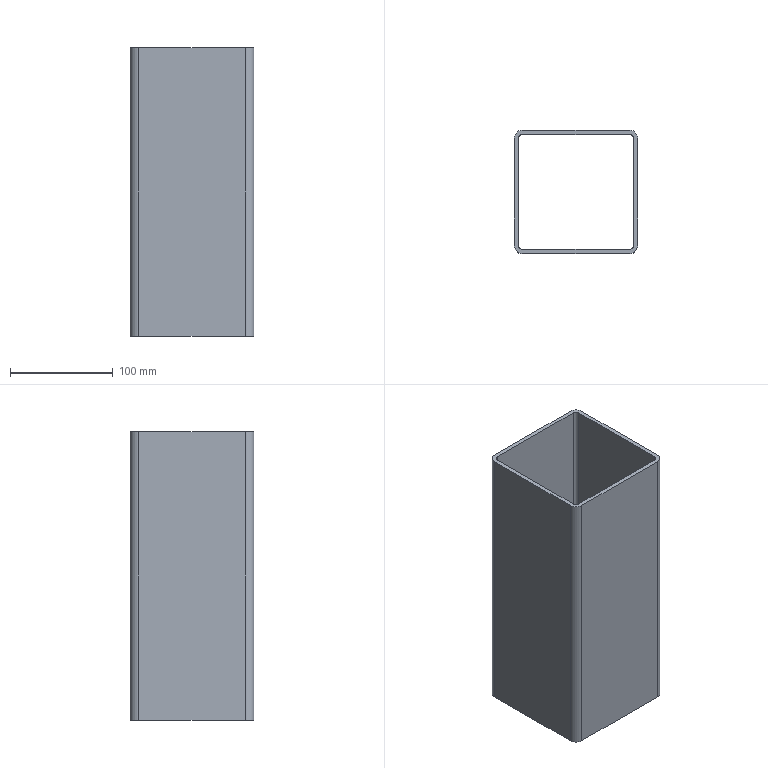Part | SolidWorks | features ICE 1, LibraryFeature 1 | 1 solid | 18 faces | box 120 x 120 x 280 mm | volume 508143 mm3 | plane 10 | cylinder 8 | commonest cylinder face diameters 8 x4 16 x4
STEP:
#1=CARTESIAN_POINT('',(52.,60.,-140.));
#2=VERTEX_POINT('',#1);
#3=CARTESIAN_POINT('',(-52.,60.,-140.));
#4=VERTEX_POINT('',#3);
#5=CARTESIAN_POINT('',(0.,60.,-140.));
#6=DIRECTION('',(-1.,0.,0.));
#7=VECTOR('',#6,1000.);
#8=LINE('',#5,#7);
#9=EDGE_CURVE('',#2,#4,#8,.T.);
#10=ORIENTED_EDGE('',*,*,#9,.T.);
#11=CARTESIAN_POINT('',(-52.,60.,140.));
#12=VERTEX_POINT('',#11);
#13=CARTESIAN_POINT('',(-52.,60.,140.));
#14=DIRECTION('',(0.,0.,-1.));
#15=VECTOR('',#14,1000.);
#16=LINE('',#13,#15);
#17=EDGE_CURVE('',#12,#4,#16,.T.);
#18=ORIENTED_EDGE('',*,*,#17,.F.);
#19=CARTESIAN_POINT('',(52.,60.,140.));
#20=VERTEX_POINT('',#19);
#21=CARTESIAN_POINT('',(0.,60.,140.));
#22=DIRECTION('',(-1.,0.,0.));
#23=VECTOR('',#22,1000.);
#24=LINE('',#21,#23);
#25=EDGE_CURVE('',#20,#12,#24,.T.);
#26=ORIENTED_EDGE('',*,*,#25,.F.);
#27=CARTESIAN_POINT('',(52.,60.,140.));
#28=DIRECTION('',(0.,0.,-1.));
#29=VECTOR('',#28,1000.);
#30=LINE('',#27,#29);
#31=EDGE_CURVE('',#20,#2,#30,.T.);
#32=ORIENTED_EDGE('',*,*,#31,.T.);
#33=EDGE_LOOP('',(#10,#18,#26,#32));
#34=FACE_OUTER_BOUND('',#33,.T.);
#35=CARTESIAN_POINT('',(0.,60.,140.));
#36=DIRECTION('',(0.,-1.,0.));
#37=DIRECTION('',(0.,0.,-1.));
#38=AXIS2_PLACEMENT_3D('',#35,#36,#37);
#39=PLANE('',#38);
#40=ADVANCED_FACE('',(#34),#39,.F.);
#41=CARTESIAN_POINT('',(-60.,52.,-140.));
#42=VERTEX_POINT('',#41);
#43=CARTESIAN_POINT('',(-52.,52.,-140.));
#44=DIRECTION('',(0.,0.,1.));
#45=DIRECTION('',(1.,0.,0.));
#46=AXIS2_PLACEMENT_3D('',#43,#44,#45);
#47=CIRCLE('',#46,8.);
#48=EDGE_CURVE('',#4,#42,#47,.T.);
#49=ORIENTED_EDGE('',*,*,#48,.T.);
#50=CARTESIAN_POINT('',(-60.,52.,140.));
#51=VERTEX_POINT('',#50);
#52=CARTESIAN_POINT('',(-60.,52.,140.));
#53=DIRECTION('',(0.,0.,-1.));
#54=VECTOR('',#53,1000.);
#55=LINE('',#52,#54);
#56=EDGE_CURVE('',#51,#42,#55,.T.);
#57=ORIENTED_EDGE('',*,*,#56,.F.);
#58=CARTESIAN_POINT('',(-52.,52.,140.));
#59=DIRECTION('',(0.,0.,1.));
#60=DIRECTION('',(1.,0.,0.));
#61=AXIS2_PLACEMENT_3D('',#58,#59,#60);
#62=CIRCLE('',#61,8.);
#63=EDGE_CURVE('',#12,#51,#62,.T.);
#64=ORIENTED_EDGE('',*,*,#63,.F.);
#65=ORIENTED_EDGE('',*,*,#17,.T.);
#66=EDGE_LOOP('',(#49,#57,#64,#65));
#67=FACE_OUTER_BOUND('',#66,.T.);
#68=CARTESIAN_POINT('',(-52.,52.,140.));
#69=DIRECTION('',(0.,0.,-1.));
#70=DIRECTION('',(-1.,0.,0.));
#71=AXIS2_PLACEMENT_3D('',#68,#69,#70);
#72=CYLINDRICAL_SURFACE('',#71,8.);
#73=ADVANCED_FACE('',(#67),#72,.T.);
#74=CARTESIAN_POINT('',(-60.,-52.,-140.));
#75=VERTEX_POINT('',#74);
#76=CARTESIAN_POINT('',(-60.,0.,-140.));
#77=DIRECTION('',(0.,1.,0.));
#78=VECTOR('',#77,1000.);
#79=LINE('',#76,#78);
#80=EDGE_CURVE('',#75,#42,#79,.T.);
#81=ORIENTED_EDGE('',*,*,#80,.F.);
#82=CARTESIAN_POINT('',(-60.,-52.,140.));
#83=VERTEX_POINT('',#82);
#84=CARTESIAN_POINT('',(-60.,-52.,140.));
#85=DIRECTION('',(0.,0.,-1.));
#86=VECTOR('',#85,1000.);
#87=LINE('',#84,#86);
#88=EDGE_CURVE('',#83,#75,#87,.T.);
#89=ORIENTED_EDGE('',*,*,#88,.F.);
#90=CARTESIAN_POINT('',(-60.,0.,140.));
#91=DIRECTION('',(0.,1.,0.));
#92=VECTOR('',#91,1000.);
#93=LINE('',#90,#92);
#94=EDGE_CURVE('',#83,#51,#93,.T.);
#95=ORIENTED_EDGE('',*,*,#94,.T.);
#96=ORIENTED_EDGE('',*,*,#56,.T.);
#97=EDGE_LOOP('',(#81,#89,#95,#96));
#98=FACE_OUTER_BOUND('',#97,.T.);
#99=CARTESIAN_POINT('',(-60.,0.,140.));
#100=DIRECTION('',(-1.,0.,0.));
#101=DIRECTION('',(0.,0.,1.));
#102=AXIS2_PLACEMENT_3D('',#99,#100,#101);
#103=PLANE('',#102);
#104=ADVANCED_FACE('',(#98),#103,.T.);
#105=CARTESIAN_POINT('',(-52.,-60.,-140.));
#106=VERTEX_POINT('',#105);
#107=CARTESIAN_POINT('',(-52.,-52.,-140.));
#108=DIRECTION('',(0.,0.,1.));
#109=DIRECTION('',(1.,0.,0.));
#110=AXIS2_PLACEMENT_3D('',#107,#108,#109);
#111=CIRCLE('',#110,8.);
#112=EDGE_CURVE('',#75,#106,#111,.T.);
#113=ORIENTED_EDGE('',*,*,#112,.T.);
#114=CARTESIAN_POINT('',(-52.,-60.,140.));
#115=VERTEX_POINT('',#114);
#116=CARTESIAN_POINT('',(-52.,-60.,140.));
#117=DIRECTION('',(0.,0.,-1.));
#118=VECTOR('',#117,1000.);
#119=LINE('',#116,#118);
#120=EDGE_CURVE('',#115,#106,#119,.T.);
#121=ORIENTED_EDGE('',*,*,#120,.F.);
#122=CARTESIAN_POINT('',(-52.,-52.,140.));
#123=DIRECTION('',(0.,0.,1.));
#124=DIRECTION('',(1.,0.,0.));
#125=AXIS2_PLACEMENT_3D('',#122,#123,#124);
#126=CIRCLE('',#125,8.);
#127=EDGE_CURVE('',#83,#115,#126,.T.);
#128=ORIENTED_EDGE('',*,*,#127,.F.);
#129=ORIENTED_EDGE('',*,*,#88,.T.);
#130=EDGE_LOOP('',(#113,#121,#128,#129));
#131=FACE_OUTER_BOUND('',#130,.T.);
#132=CARTESIAN_POINT('',(-52.,-52.,140.));
#133=DIRECTION('',(0.,0.,-1.));
#134=DIRECTION('',(-1.,0.,0.));
#135=AXIS2_PLACEMENT_3D('',#132,#133,#134);
#136=CYLINDRICAL_SURFACE('',#135,8.);
#137=ADVANCED_FACE('',(#131),#136,.T.);
#138=CARTESIAN_POINT('',(52.,-60.,-140.));
#139=VERTEX_POINT('',#138);
#140=CARTESIAN_POINT('',(0.,-60.,-140.));
#141=DIRECTION('',(1.,0.,0.));
#142=VECTOR('',#141,1000.);
#143=LINE('',#140,#142);
#144=EDGE_CURVE('',#106,#139,#143,.T.);
#145=ORIENTED_EDGE('',*,*,#144,.T.);
#146=CARTESIAN_POINT('',(52.,-60.,140.));
#147=VERTEX_POINT('',#146);
#148=CARTESIAN_POINT('',(52.,-60.,140.));
#149=DIRECTION('',(0.,0.,-1.));
#150=VECTOR('',#149,1000.);
#151=LINE('',#148,#150);
#152=EDGE_CURVE('',#147,#139,#151,.T.);
#153=ORIENTED_EDGE('',*,*,#152,.F.);
#154=CARTESIAN_POINT('',(0.,-60.,140.));
#155=DIRECTION('',(1.,0.,0.));
#156=VECTOR('',#155,1000.);
#157=LINE('',#154,#156);
#158=EDGE_CURVE('',#115,#147,#157,.T.);
#159=ORIENTED_EDGE('',*,*,#158,.F.);
#160=ORIENTED_EDGE('',*,*,#120,.T.);
#161=EDGE_LOOP('',(#145,#153,#159,#160));
#162=FACE_OUTER_BOUND('',#161,.T.);
#163=CARTESIAN_POINT('',(0.,-60.,140.));
#164=DIRECTION('',(0.,1.,0.));
#165=DIRECTION('',(0.,0.,1.));
#166=AXIS2_PLACEMENT_3D('',#163,#164,#165);
#167=PLANE('',#166);
#168=ADVANCED_FACE('',(#162),#167,.F.);
#169=CARTESIAN_POINT('',(60.,-52.,-140.));
#170=VERTEX_POINT('',#169);
#171=CARTESIAN_POINT('',(52.,-52.,-140.));
#172=DIRECTION('',(0.,0.,1.));
#173=DIRECTION('',(1.,0.,0.));
#174=AXIS2_PLACEMENT_3D('',#171,#172,#173);
#175=CIRCLE('',#174,8.);
#176=EDGE_CURVE('',#139,#170,#175,.T.);
#177=ORIENTED_EDGE('',*,*,#176,.T.);
#178=CARTESIAN_POINT('',(60.,-52.,140.));
#179=VERTEX_POINT('',#178);
#180=CARTESIAN_POINT('',(60.,-52.,140.));
#181=DIRECTION('',(0.,0.,-1.));
#182=VECTOR('',#181,1000.);
#183=LINE('',#180,#182);
#184=EDGE_CURVE('',#179,#170,#183,.T.);
#185=ORIENTED_EDGE('',*,*,#184,.F.);
#186=CARTESIAN_POINT('',(52.,-52.,140.));
#187=DIRECTION('',(0.,0.,1.));
#188=DIRECTION('',(1.,0.,0.));
#189=AXIS2_PLACEMENT_3D('',#186,#187,#188);
#190=CIRCLE('',#189,8.);
#191=EDGE_CURVE('',#147,#179,#190,.T.);
#192=ORIENTED_EDGE('',*,*,#191,.F.);
#193=ORIENTED_EDGE('',*,*,#152,.T.);
#194=EDGE_LOOP('',(#177,#185,#192,#193));
#195=FACE_OUTER_BOUND('',#194,.T.);
#196=CARTESIAN_POINT('',(52.,-52.,140.));
#197=DIRECTION('',(0.,0.,-1.));
#198=DIRECTION('',(-1.,0.,0.));
#199=AXIS2_PLACEMENT_3D('',#196,#197,#198);
#200=CYLINDRICAL_SURFACE('',#199,8.);
#201=ADVANCED_FACE('',(#195),#200,.T.);
#202=CARTESIAN_POINT('',(60.,52.,-140.));
#203=VERTEX_POINT('',#202);
#204=CARTESIAN_POINT('',(60.,0.,-140.));
#205=DIRECTION('',(0.,-1.,0.));
#206=VECTOR('',#205,1000.);
#207=LINE('',#204,#206);
#208=EDGE_CURVE('',#203,#170,#207,.T.);
#209=ORIENTED_EDGE('',*,*,#208,.F.);
#210=CARTESIAN_POINT('',(60.,52.,140.));
#211=VERTEX_POINT('',#210);
#212=CARTESIAN_POINT('',(60.,52.,140.));
#213=DIRECTION('',(0.,0.,-1.));
#214=VECTOR('',#213,1000.);
#215=LINE('',#212,#214);
#216=EDGE_CURVE('',#211,#203,#215,.T.);
#217=ORIENTED_EDGE('',*,*,#216,.F.);
#218=CARTESIAN_POINT('',(60.,0.,140.));
#219=DIRECTION('',(0.,-1.,0.));
#220=VECTOR('',#219,1000.);
#221=LINE('',#218,#220);
#222=EDGE_CURVE('',#211,#179,#221,.T.);
#223=ORIENTED_EDGE('',*,*,#222,.T.);
#224=ORIENTED_EDGE('',*,*,#184,.T.);
#225=EDGE_LOOP('',(#209,#217,#223,#224));
#226=FACE_OUTER_BOUND('',#225,.T.);
#227=CARTESIAN_POINT('',(60.,0.,140.));
#228=DIRECTION('',(1.,0.,0.));
#229=DIRECTION('',(0.,0.,-1.));
#230=AXIS2_PLACEMENT_3D('',#227,#228,#229);
#231=PLANE('',#230);
#232=ADVANCED_FACE('',(#226),#231,.T.);
#233=CARTESIAN_POINT('',(-56.,-52.,-140.));
#234=VERTEX_POINT('',#233);
#235=CARTESIAN_POINT('',(-52.,-56.,-140.));
#236=VERTEX_POINT('',#235);
#237=CARTESIAN_POINT('',(-52.,-52.,-140.));
#238=DIRECTION('',(0.,0.,1.));
#239=DIRECTION('',(1.,0.,0.));
#240=AXIS2_PLACEMENT_3D('',#237,#238,#239);
#241=CIRCLE('',#240,4.);
#242=EDGE_CURVE('',#234,#236,#241,.T.);
#243=ORIENTED_EDGE('',*,*,#242,.F.);
#244=CARTESIAN_POINT('',(-56.,-52.,140.));
#245=VERTEX_POINT('',#244);
#246=CARTESIAN_POINT('',(-56.,-52.,140.));
#247=DIRECTION('',(0.,0.,-1.));
#248=VECTOR('',#247,1000.);
#249=LINE('',#246,#248);
#250=EDGE_CURVE('',#245,#234,#249,.T.);
#251=ORIENTED_EDGE('',*,*,#250,.F.);
#252=CARTESIAN_POINT('',(-52.,-56.,140.));
#253=VERTEX_POINT('',#252);
#254=CARTESIAN_POINT('',(-52.,-52.,140.));
#255=DIRECTION('',(0.,0.,1.));
#256=DIRECTION('',(1.,0.,0.));
#257=AXIS2_PLACEMENT_3D('',#254,#255,#256);
#258=CIRCLE('',#257,4.);
#259=EDGE_CURVE('',#245,#253,#258,.T.);
#260=ORIENTED_EDGE('',*,*,#259,.T.);
#261=CARTESIAN_POINT('',(-52.,-56.,140.));
#262=DIRECTION('',(0.,0.,-1.));
#263=VECTOR('',#262,1000.);
#264=LINE('',#261,#263);
#265=EDGE_CURVE('',#253,#236,#264,.T.);
#266=ORIENTED_EDGE('',*,*,#265,.T.);
#267=EDGE_LOOP('',(#243,#251,#260,#266));
#268=FACE_OUTER_BOUND('',#267,.T.);
#269=CARTESIAN_POINT('',(-52.,-52.,140.));
#270=DIRECTION('',(0.,0.,-1.));
#271=DIRECTION('',(-1.,0.,0.));
#272=AXIS2_PLACEMENT_3D('',#269,#270,#271);
#273=CYLINDRICAL_SURFACE('',#272,4.);
#274=ADVANCED_FACE('',(#268),#273,.F.);
#275=CARTESIAN_POINT('',(-56.,52.,-140.));
#276=VERTEX_POINT('',#275);
#277=CARTESIAN_POINT('',(-56.,0.,-140.));
#278=DIRECTION('',(0.,1.,0.));
#279=VECTOR('',#278,1000.);
#280=LINE('',#277,#279);
#281=EDGE_CURVE('',#234,#276,#280,.T.);
#282=ORIENTED_EDGE('',*,*,#281,.T.);
#283=CARTESIAN_POINT('',(-56.,52.,140.));
#284=VERTEX_POINT('',#283);
#285=CARTESIAN_POINT('',(-56.,52.,140.));
#286=DIRECTION('',(0.,0.,-1.));
#287=VECTOR('',#286,1000.);
#288=LINE('',#285,#287);
#289=EDGE_CURVE('',#284,#276,#288,.T.);
#290=ORIENTED_EDGE('',*,*,#289,.F.);
#291=CARTESIAN_POINT('',(-56.,0.,140.));
#292=DIRECTION('',(0.,1.,0.));
#293=VECTOR('',#292,1000.);
#294=LINE('',#291,#293);
#295=EDGE_CURVE('',#245,#284,#294,.T.);
#296=ORIENTED_EDGE('',*,*,#295,.F.);
#297=ORIENTED_EDGE('',*,*,#250,.T.);
#298=EDGE_LOOP('',(#282,#290,#296,#297));
#299=FACE_OUTER_BOUND('',#298,.T.);
#300=CARTESIAN_POINT('',(-56.,0.,140.));
#301=DIRECTION('',(-1.,0.,0.));
#302=DIRECTION('',(0.,0.,1.));
#303=AXIS2_PLACEMENT_3D('',#300,#301,#302);
#304=PLANE('',#303);
#305=ADVANCED_FACE('',(#299),#304,.F.);
#306=CARTESIAN_POINT('',(-52.,56.,-140.));
#307=VERTEX_POINT('',#306);
#308=CARTESIAN_POINT('',(-52.,52.,-140.));
#309=DIRECTION('',(0.,0.,1.));
#310=DIRECTION('',(1.,0.,0.));
#311=AXIS2_PLACEMENT_3D('',#308,#309,#310);
#312=CIRCLE('',#311,4.);
#313=EDGE_CURVE('',#307,#276,#312,.T.);
#314=ORIENTED_EDGE('',*,*,#313,.F.);
#315=CARTESIAN_POINT('',(-52.,56.,140.));
#316=VERTEX_POINT('',#315);
#317=CARTESIAN_POINT('',(-52.,56.,140.));
#318=DIRECTION('',(0.,0.,-1.));
#319=VECTOR('',#318,1000.);
#320=LINE('',#317,#319);
#321=EDGE_CURVE('',#316,#307,#320,.T.);
#322=ORIENTED_EDGE('',*,*,#321,.F.);
#323=CARTESIAN_POINT('',(-52.,52.,140.));
#324=DIRECTION('',(0.,0.,1.));
#325=DIRECTION('',(1.,0.,0.));
#326=AXIS2_PLACEMENT_3D('',#323,#324,#325);
#327=CIRCLE('',#326,4.);
#328=EDGE_CURVE('',#316,#284,#327,.T.);
#329=ORIENTED_EDGE('',*,*,#328,.T.);
#330=ORIENTED_EDGE('',*,*,#289,.T.);
#331=EDGE_LOOP('',(#314,#322,#329,#330));
#332=FACE_OUTER_BOUND('',#331,.T.);
#333=CARTESIAN_POINT('',(-52.,52.,140.));
#334=DIRECTION('',(0.,0.,-1.));
#335=DIRECTION('',(-1.,0.,0.));
#336=AXIS2_PLACEMENT_3D('',#333,#334,#335);
#337=CYLINDRICAL_SURFACE('',#336,4.);
#338=ADVANCED_FACE('',(#332),#337,.F.);
#339=CARTESIAN_POINT('',(52.,56.,-140.));
#340=VERTEX_POINT('',#339);
#341=CARTESIAN_POINT('',(0.,56.,-140.));
#342=DIRECTION('',(-1.,0.,0.));
#343=VECTOR('',#342,1000.);
#344=LINE('',#341,#343);
#345=EDGE_CURVE('',#340,#307,#344,.T.);
#346=ORIENTED_EDGE('',*,*,#345,.F.);
#347=CARTESIAN_POINT('',(52.,56.,140.));
#348=VERTEX_POINT('',#347);
#349=CARTESIAN_POINT('',(52.,56.,140.));
#350=DIRECTION('',(0.,0.,-1.));
#351=VECTOR('',#350,1000.);
#352=LINE('',#349,#351);
#353=EDGE_CURVE('',#348,#340,#352,.T.);
#354=ORIENTED_EDGE('',*,*,#353,.F.);
#355=CARTESIAN_POINT('',(0.,56.,140.));
#356=DIRECTION('',(-1.,0.,0.));
#357=VECTOR('',#356,1000.);
#358=LINE('',#355,#357);
#359=EDGE_CURVE('',#348,#316,#358,.T.);
#360=ORIENTED_EDGE('',*,*,#359,.T.);
#361=ORIENTED_EDGE('',*,*,#321,.T.);
#362=EDGE_LOOP('',(#346,#354,#360,#361));
#363=FACE_OUTER_BOUND('',#362,.T.);
#364=CARTESIAN_POINT('',(0.,56.,140.));
#365=DIRECTION('',(0.,-1.,0.));
#366=DIRECTION('',(0.,0.,-1.));
#367=AXIS2_PLACEMENT_3D('',#364,#365,#366);
#368=PLANE('',#367);
#369=ADVANCED_FACE('',(#363),#368,.T.);
#370=CARTESIAN_POINT('',(56.,52.,-140.));
#371=VERTEX_POINT('',#370);
#372=CARTESIAN_POINT('',(52.,52.,-140.));
#373=DIRECTION('',(0.,0.,1.));
#374=DIRECTION('',(1.,0.,0.));
#375=AXIS2_PLACEMENT_3D('',#372,#373,#374);
#376=CIRCLE('',#375,4.);
#377=EDGE_CURVE('',#371,#340,#376,.T.);
#378=ORIENTED_EDGE('',*,*,#377,.F.);
#379=CARTESIAN_POINT('',(56.,52.,140.));
#380=VERTEX_POINT('',#379);
#381=CARTESIAN_POINT('',(56.,52.,140.));
#382=DIRECTION('',(0.,0.,-1.));
#383=VECTOR('',#382,1000.);
#384=LINE('',#381,#383);
#385=EDGE_CURVE('',#380,#371,#384,.T.);
#386=ORIENTED_EDGE('',*,*,#385,.F.);
#387=CARTESIAN_POINT('',(52.,52.,140.));
#388=DIRECTION('',(0.,0.,1.));
#389=DIRECTION('',(1.,0.,0.));
#390=AXIS2_PLACEMENT_3D('',#387,#388,#389);
#391=CIRCLE('',#390,4.);
#392=EDGE_CURVE('',#380,#348,#391,.T.);
#393=ORIENTED_EDGE('',*,*,#392,.T.);
#394=ORIENTED_EDGE('',*,*,#353,.T.);
#395=EDGE_LOOP('',(#378,#386,#393,#394));
#396=FACE_OUTER_BOUND('',#395,.T.);
#397=CARTESIAN_POINT('',(52.,52.,140.));
#398=DIRECTION('',(0.,0.,-1.));
#399=DIRECTION('',(-1.,0.,0.));
#400=AXIS2_PLACEMENT_3D('',#397,#398,#399);
#401=CYLINDRICAL_SURFACE('',#400,4.);
#402=ADVANCED_FACE('',(#396),#401,.F.);
#403=CARTESIAN_POINT('',(56.,-52.,-140.));
#404=VERTEX_POINT('',#403);
#405=CARTESIAN_POINT('',(56.,0.,-140.));
#406=DIRECTION('',(0.,-1.,0.));
#407=VECTOR('',#406,1000.);
#408=LINE('',#405,#407);
#409=EDGE_CURVE('',#371,#404,#408,.T.);
#410=ORIENTED_EDGE('',*,*,#409,.T.);
#411=CARTESIAN_POINT('',(56.,-52.,140.));
#412=VERTEX_POINT('',#411);
#413=CARTESIAN_POINT('',(56.,-52.,140.));
#414=DIRECTION('',(0.,0.,-1.));
#415=VECTOR('',#414,1000.);
#416=LINE('',#413,#415);
#417=EDGE_CURVE('',#412,#404,#416,.T.);
#418=ORIENTED_EDGE('',*,*,#417,.F.);
#419=CARTESIAN_POINT('',(56.,0.,140.));
#420=DIRECTION('',(0.,-1.,0.));
#421=VECTOR('',#420,1000.);
#422=LINE('',#419,#421);
#423=EDGE_CURVE('',#380,#412,#422,.T.);
#424=ORIENTED_EDGE('',*,*,#423,.F.);
#425=ORIENTED_EDGE('',*,*,#385,.T.);
#426=EDGE_LOOP('',(#410,#418,#424,#425));
#427=FACE_OUTER_BOUND('',#426,.T.);
#428=CARTESIAN_POINT('',(56.,0.,140.));
#429=DIRECTION('',(1.,0.,0.));
#430=DIRECTION('',(0.,0.,-1.));
#431=AXIS2_PLACEMENT_3D('',#428,#429,#430);
#432=PLANE('',#431);
#433=ADVANCED_FACE('',(#427),#432,.F.);
#434=CARTESIAN_POINT('',(52.,-56.,-140.));
#435=VERTEX_POINT('',#434);
#436=CARTESIAN_POINT('',(52.,-52.,-140.));
#437=DIRECTION('',(0.,0.,1.));
#438=DIRECTION('',(1.,0.,0.));
#439=AXIS2_PLACEMENT_3D('',#436,#437,#438);
#440=CIRCLE('',#439,4.);
#441=EDGE_CURVE('',#435,#404,#440,.T.);
#442=ORIENTED_EDGE('',*,*,#441,.F.);
#443=CARTESIAN_POINT('',(52.,-56.,140.));
#444=VERTEX_POINT('',#443);
#445=CARTESIAN_POINT('',(52.,-56.,140.));
#446=DIRECTION('',(0.,0.,-1.));
#447=VECTOR('',#446,1000.);
#448=LINE('',#445,#447);
#449=EDGE_CURVE('',#444,#435,#448,.T.);
#450=ORIENTED_EDGE('',*,*,#449,.F.);
#451=CARTESIAN_POINT('',(52.,-52.,140.));
#452=DIRECTION('',(0.,0.,1.));
#453=DIRECTION('',(1.,0.,0.));
#454=AXIS2_PLACEMENT_3D('',#451,#452,#453);
#455=CIRCLE('',#454,4.);
#456=EDGE_CURVE('',#444,#412,#455,.T.);
#457=ORIENTED_EDGE('',*,*,#456,.T.);
#458=ORIENTED_EDGE('',*,*,#417,.T.);
#459=EDGE_LOOP('',(#442,#450,#457,#458));
#460=FACE_OUTER_BOUND('',#459,.T.);
#461=CARTESIAN_POINT('',(52.,-52.,140.));
#462=DIRECTION('',(0.,0.,-1.));
#463=DIRECTION('',(-1.,0.,0.));
#464=AXIS2_PLACEMENT_3D('',#461,#462,#463);
#465=CYLINDRICAL_SURFACE('',#464,4.);
#466=ADVANCED_FACE('',(#460),#465,.F.);
#467=CARTESIAN_POINT('',(0.,-56.,-140.));
#468=DIRECTION('',(1.,0.,0.));
#469=VECTOR('',#468,1000.);
#470=LINE('',#467,#469);
#471=EDGE_CURVE('',#236,#435,#470,.T.);
#472=ORIENTED_EDGE('',*,*,#471,.F.);
#473=ORIENTED_EDGE('',*,*,#265,.F.);
#474=CARTESIAN_POINT('',(0.,-56.,140.));
#475=DIRECTION('',(1.,0.,0.));
#476=VECTOR('',#475,1000.);
#477=LINE('',#474,#476);
#478=EDGE_CURVE('',#253,#444,#477,.T.);
#479=ORIENTED_EDGE('',*,*,#478,.T.);
#480=ORIENTED_EDGE('',*,*,#449,.T.);
#481=EDGE_LOOP('',(#472,#473,#479,#480));
#482=FACE_OUTER_BOUND('',#481,.T.);
#483=CARTESIAN_POINT('',(0.,-56.,140.));
#484=DIRECTION('',(0.,1.,0.));
#485=DIRECTION('',(0.,0.,1.));
#486=AXIS2_PLACEMENT_3D('',#483,#484,#485);
#487=PLANE('',#486);
#488=ADVANCED_FACE('',(#482),#487,.T.);
#489=CARTESIAN_POINT('',(52.,52.,-140.));
#490=DIRECTION('',(0.,0.,1.));
#491=DIRECTION('',(1.,0.,0.));
#492=AXIS2_PLACEMENT_3D('',#489,#490,#491);
#493=CIRCLE('',#492,8.);
#494=EDGE_CURVE('',#203,#2,#493,.T.);
#495=ORIENTED_EDGE('',*,*,#494,.T.);
#496=ORIENTED_EDGE('',*,*,#31,.F.);
#497=CARTESIAN_POINT('',(52.,52.,140.));
#498=DIRECTION('',(0.,0.,1.));
#499=DIRECTION('',(1.,0.,0.));
#500=AXIS2_PLACEMENT_3D('',#497,#498,#499);
#501=CIRCLE('',#500,8.);
#502=EDGE_CURVE('',#211,#20,#501,.T.);
#503=ORIENTED_EDGE('',*,*,#502,.F.);
#504=ORIENTED_EDGE('',*,*,#216,.T.);
#505=EDGE_LOOP('',(#495,#496,#503,#504));
#506=FACE_OUTER_BOUND('',#505,.T.);
#507=CARTESIAN_POINT('',(52.,52.,140.));
#508=DIRECTION('',(0.,0.,-1.));
#509=DIRECTION('',(-1.,0.,0.));
#510=AXIS2_PLACEMENT_3D('',#507,#508,#509);
#511=CYLINDRICAL_SURFACE('',#510,8.);
#512=ADVANCED_FACE('',(#506),#511,.T.);
#513=ORIENTED_EDGE('',*,*,#259,.F.);
#514=ORIENTED_EDGE('',*,*,#295,.T.);
#515=ORIENTED_EDGE('',*,*,#328,.F.);
#516=ORIENTED_EDGE('',*,*,#359,.F.);
#517=ORIENTED_EDGE('',*,*,#392,.F.);
#518=ORIENTED_EDGE('',*,*,#423,.T.);
#519=ORIENTED_EDGE('',*,*,#456,.F.);
#520=ORIENTED_EDGE('',*,*,#478,.F.);
#521=EDGE_LOOP('',(#513,#514,#515,#516,#517,#518,#519,#520));
#522=FACE_BOUND('',#521,.T.);
#523=ORIENTED_EDGE('',*,*,#25,.T.);
#524=ORIENTED_EDGE('',*,*,#63,.T.);
#525=ORIENTED_EDGE('',*,*,#94,.F.);
#526=ORIENTED_EDGE('',*,*,#127,.T.);
#527=ORIENTED_EDGE('',*,*,#158,.T.);
#528=ORIENTED_EDGE('',*,*,#191,.T.);
#529=ORIENTED_EDGE('',*,*,#222,.F.);
#530=ORIENTED_EDGE('',*,*,#502,.T.);
#531=EDGE_LOOP('',(#523,#524,#525,#526,#527,#528,#529,#530));
#532=FACE_OUTER_BOUND('',#531,.T.);
#533=CARTESIAN_POINT('',(0.,0.,140.));
#534=DIRECTION('',(0.,0.,1.));
#535=DIRECTION('',(1.,0.,0.));
#536=AXIS2_PLACEMENT_3D('',#533,#534,#535);
#537=PLANE('',#536);
#538=ADVANCED_FACE('',(#522,#532),#537,.T.);
#539=ORIENTED_EDGE('',*,*,#242,.T.);
#540=ORIENTED_EDGE('',*,*,#471,.T.);
#541=ORIENTED_EDGE('',*,*,#441,.T.);
#542=ORIENTED_EDGE('',*,*,#409,.F.);
#543=ORIENTED_EDGE('',*,*,#377,.T.);
#544=ORIENTED_EDGE('',*,*,#345,.T.);
#545=ORIENTED_EDGE('',*,*,#313,.T.);
#546=ORIENTED_EDGE('',*,*,#281,.F.);
#547=EDGE_LOOP('',(#539,#540,#541,#542,#543,#544,#545,#546));
#548=FACE_BOUND('',#547,.T.);
#549=ORIENTED_EDGE('',*,*,#9,.F.);
#550=ORIENTED_EDGE('',*,*,#494,.F.);
#551=ORIENTED_EDGE('',*,*,#208,.T.);
#552=ORIENTED_EDGE('',*,*,#176,.F.);
#553=ORIENTED_EDGE('',*,*,#144,.F.);
#554=ORIENTED_EDGE('',*,*,#112,.F.);
#555=ORIENTED_EDGE('',*,*,#80,.T.);
#556=ORIENTED_EDGE('',*,*,#48,.F.);
#557=EDGE_LOOP('',(#549,#550,#551,#552,#553,#554,#555,#556));
#558=FACE_OUTER_BOUND('',#557,.T.);
#559=CARTESIAN_POINT('',(0.,0.,-140.));
#560=DIRECTION('',(0.,0.,1.));
#561=DIRECTION('',(1.,0.,0.));
#562=AXIS2_PLACEMENT_3D('',#559,#560,#561);
#563=PLANE('',#562);
#564=ADVANCED_FACE('',(#548,#558),#563,.F.);
#565=CLOSED_SHELL('',(#40,#73,#104,#137,#168,#201,#232,#274,#305,#338,#369,#402,#433,#466,#488,#512,#538,#564));
#566=MANIFOLD_SOLID_BREP('',#565);
#567=CARTESIAN_POINT('',(0.,0.,0.));
#568=DIRECTION('',(0.,0.,1.));
#569=DIRECTION('',(1.,0.,0.));
#570=AXIS2_PLACEMENT_3D('',#567,#568,#569);
#571=(LENGTH_UNIT()NAMED_UNIT(*)SI_UNIT(.MILLI.,.METRE.));
#572=UNCERTAINTY_MEASURE_WITH_UNIT(LENGTH_MEASURE(0.00001),#571,'','');
#573=(NAMED_UNIT(*)PLANE_ANGLE_UNIT()SI_UNIT($,.RADIAN.));
#574=(NAMED_UNIT(*)SI_UNIT($,.STERADIAN.)SOLID_ANGLE_UNIT());
#575=(GEOMETRIC_REPRESENTATION_CONTEXT(3)GLOBAL_UNCERTAINTY_ASSIGNED_CONTEXT((#572))GLOBAL_UNIT_ASSIGNED_CONTEXT((#571,#573,#574))REPRESENTATION_CONTEXT('',''));
#576=ADVANCED_BREP_SHAPE_REPRESENTATION('',(#566,#570),#575);